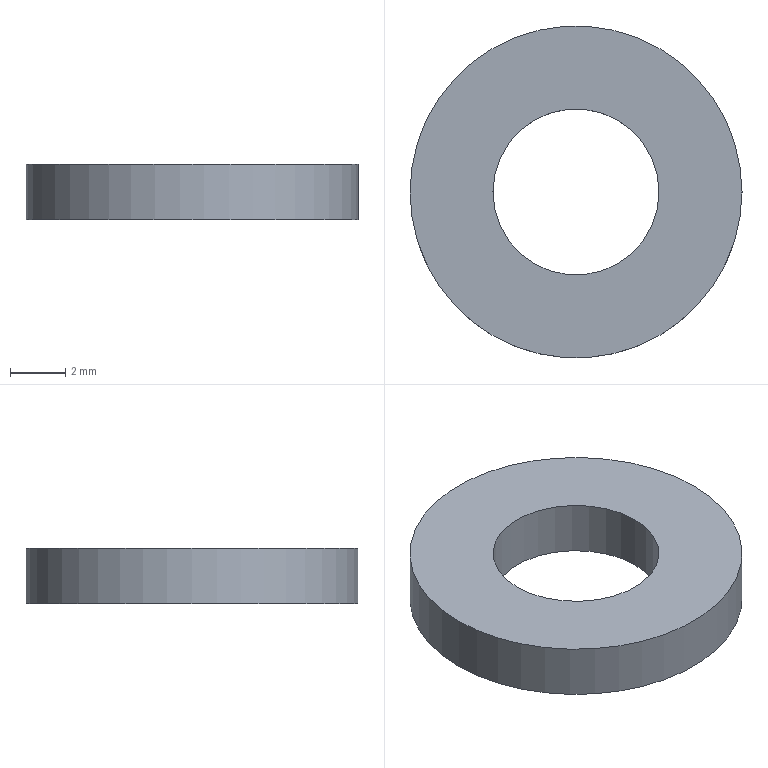Part | STEP file | 1-S938U-100524-008 | 1 solid | 4 faces | box 12 x 12 x 2 mm | volume 169.646 mm3 | cylinder 2 | plane 2 | commonest cylinder face diameters 6 x1 12 x1
STEP:
#1=CARTESIAN_POINT('',(3.,0.,0.));
#2=VERTEX_POINT('',#1);
#3=CARTESIAN_POINT('',(0.,0.,0.));
#4=DIRECTION('',(0.,0.,-1.));
#5=DIRECTION('',(-1.,0.,0.));
#6=AXIS2_PLACEMENT_3D('',#3,#4,#5);
#7=CIRCLE('',#6,3.);
#8=EDGE_CURVE('',#2,#2,#7,.T.);
#9=ORIENTED_EDGE('',*,*,#8,.T.);
#10=CARTESIAN_POINT('',(3.,0.,2.));
#11=VERTEX_POINT('',#10);
#12=CARTESIAN_POINT('',(3.,0.,0.));
#13=DIRECTION('',(0.,0.,1.));
#14=VECTOR('',#13,3.);
#15=LINE('',#12,#14);
#16=EDGE_CURVE('',#2,#11,#15,.T.);
#17=ORIENTED_EDGE('',*,*,#16,.T.);
#18=CARTESIAN_POINT('',(0.,0.,2.));
#19=DIRECTION('',(0.,0.,-1.));
#20=DIRECTION('',(-1.,0.,0.));
#21=AXIS2_PLACEMENT_3D('',#18,#19,#20);
#22=CIRCLE('',#21,3.);
#23=EDGE_CURVE('',#11,#11,#22,.T.);
#24=ORIENTED_EDGE('',*,*,#23,.F.);
#25=ORIENTED_EDGE('',*,*,#16,.F.);
#26=EDGE_LOOP('',(#9,#17,#24,#25));
#27=FACE_OUTER_BOUND('',#26,.T.);
#28=CARTESIAN_POINT('',(0.,0.,0.));
#29=DIRECTION('',(0.,0.,1.));
#30=DIRECTION('',(-1.,0.,0.));
#31=AXIS2_PLACEMENT_3D('',#28,#29,#30);
#32=CYLINDRICAL_SURFACE('',#31,3.);
#33=ADVANCED_FACE('',(#27),#32,.F.);
#34=CARTESIAN_POINT('',(6.,0.,2.));
#35=VERTEX_POINT('',#34);
#36=CARTESIAN_POINT('',(-6.,0.,2.));
#37=VERTEX_POINT('',#36);
#38=CARTESIAN_POINT('',(0.,0.,2.));
#39=DIRECTION('',(0.,0.,1.));
#40=DIRECTION('',(1.,0.,0.));
#41=AXIS2_PLACEMENT_3D('',#38,#39,#40);
#42=CIRCLE('',#41,6.);
#43=EDGE_CURVE('',#35,#37,#42,.T.);
#44=ORIENTED_EDGE('',*,*,#43,.F.);
#45=CARTESIAN_POINT('',(0.,0.,2.));
#46=DIRECTION('',(0.,0.,1.));
#47=DIRECTION('',(1.,0.,0.));
#48=AXIS2_PLACEMENT_3D('',#45,#46,#47);
#49=CIRCLE('',#48,6.);
#50=EDGE_CURVE('',#37,#35,#49,.T.);
#51=ORIENTED_EDGE('',*,*,#50,.F.);
#52=CARTESIAN_POINT('',(-6.,0.,0.));
#53=VERTEX_POINT('',#52);
#54=CARTESIAN_POINT('',(-6.,0.,0.));
#55=DIRECTION('',(0.,0.,-1.));
#56=VECTOR('',#55,6.);
#57=LINE('',#54,#56);
#58=EDGE_CURVE('',#37,#53,#57,.T.);
#59=ORIENTED_EDGE('',*,*,#58,.T.);
#60=CARTESIAN_POINT('',(6.,0.,0.));
#61=VERTEX_POINT('',#60);
#62=CARTESIAN_POINT('',(0.,0.,0.));
#63=DIRECTION('',(0.,0.,1.));
#64=DIRECTION('',(1.,0.,0.));
#65=AXIS2_PLACEMENT_3D('',#62,#63,#64);
#66=CIRCLE('',#65,6.);
#67=EDGE_CURVE('',#53,#61,#66,.T.);
#68=ORIENTED_EDGE('',*,*,#67,.T.);
#69=CARTESIAN_POINT('',(0.,0.,0.));
#70=DIRECTION('',(0.,0.,1.));
#71=DIRECTION('',(1.,0.,0.));
#72=AXIS2_PLACEMENT_3D('',#69,#70,#71);
#73=CIRCLE('',#72,6.);
#74=EDGE_CURVE('',#61,#53,#73,.T.);
#75=ORIENTED_EDGE('',*,*,#74,.T.);
#76=ORIENTED_EDGE('',*,*,#58,.F.);
#77=EDGE_LOOP('',(#44,#51,#59,#68,#75,#76));
#78=FACE_OUTER_BOUND('',#77,.T.);
#79=CARTESIAN_POINT('',(0.,0.,0.));
#80=DIRECTION('',(0.,0.,1.));
#81=DIRECTION('',(1.,0.,0.));
#82=AXIS2_PLACEMENT_3D('',#79,#80,#81);
#83=CYLINDRICAL_SURFACE('',#82,6.);
#84=ADVANCED_FACE('',(#78),#83,.T.);
#85=ORIENTED_EDGE('',*,*,#43,.T.);
#86=ORIENTED_EDGE('',*,*,#50,.T.);
#87=EDGE_LOOP('',(#85,#86));
#88=FACE_OUTER_BOUND('',#87,.T.);
#89=ORIENTED_EDGE('',*,*,#23,.T.);
#90=EDGE_LOOP('',(#89));
#91=FACE_BOUND('',#90,.T.);
#92=CARTESIAN_POINT('',(0.,0.,2.));
#93=DIRECTION('',(0.,0.,1.));
#94=DIRECTION('',(1.,0.,0.));
#95=AXIS2_PLACEMENT_3D('',#92,#93,#94);
#96=PLANE('',#95);
#97=ADVANCED_FACE('',(#88,#91),#96,.T.);
#98=ORIENTED_EDGE('',*,*,#74,.F.);
#99=ORIENTED_EDGE('',*,*,#67,.F.);
#100=EDGE_LOOP('',(#98,#99));
#101=FACE_OUTER_BOUND('',#100,.T.);
#102=ORIENTED_EDGE('',*,*,#8,.F.);
#103=EDGE_LOOP('',(#102));
#104=FACE_BOUND('',#103,.T.);
#105=CARTESIAN_POINT('',(0.,0.,0.));
#106=DIRECTION('',(0.,0.,1.));
#107=DIRECTION('',(1.,0.,0.));
#108=AXIS2_PLACEMENT_3D('',#105,#106,#107);
#109=PLANE('',#108);
#110=ADVANCED_FACE('',(#101,#104),#109,.F.);
#111=CLOSED_SHELL('',(#33,#84,#97,#110));
#112=MANIFOLD_SOLID_BREP('',#111);
#113=(LENGTH_UNIT()NAMED_UNIT(*)SI_UNIT(.MILLI.,.METRE.));
#114=UNCERTAINTY_MEASURE_WITH_UNIT(LENGTH_MEASURE(0.01),#113,'','');
#115=(NAMED_UNIT(*)PLANE_ANGLE_UNIT()SI_UNIT($,.RADIAN.));
#116=(NAMED_UNIT(*)SI_UNIT($,.STERADIAN.)SOLID_ANGLE_UNIT());
#117=(GEOMETRIC_REPRESENTATION_CONTEXT(3)GLOBAL_UNCERTAINTY_ASSIGNED_CONTEXT((#114))GLOBAL_UNIT_ASSIGNED_CONTEXT((#113,#115,#116))REPRESENTATION_CONTEXT('',''));
#118=ADVANCED_BREP_SHAPE_REPRESENTATION('',(#112),#117);